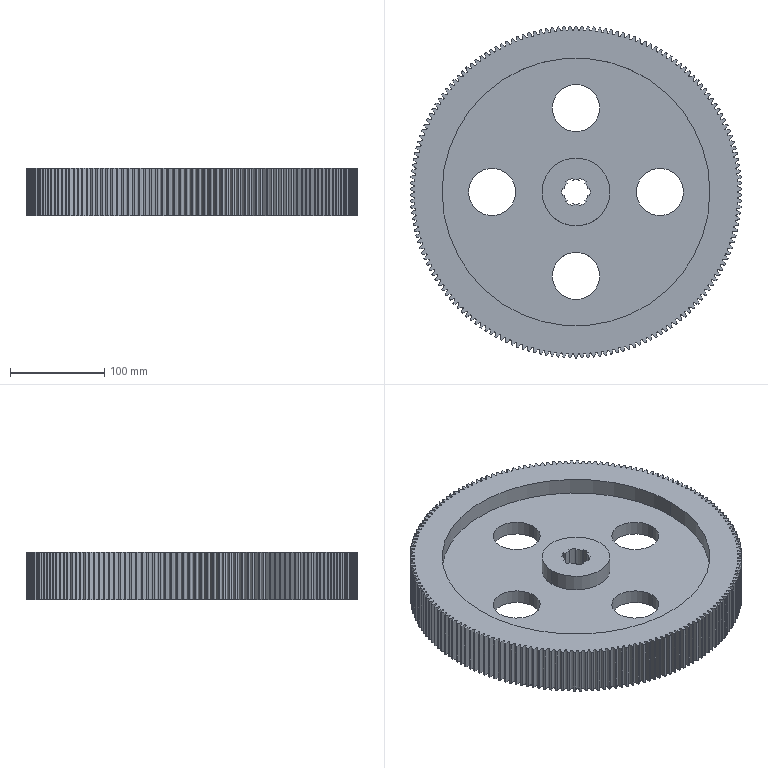Part | SolidWorks | features ICE 5, CirPattern 1, MirrorPattern 1, RefAxis 1, RevCut 1, Revolution 1 | 1 solid | 401 faces | box 351.968 x 352 x 50 mm | volume 2206869 mm3 | cylinder 207 | spline 174 | plane 20 | commonest cylinder face diameters 352 x174 50 x8 30 x7 26 x6 7 x4 72 x4